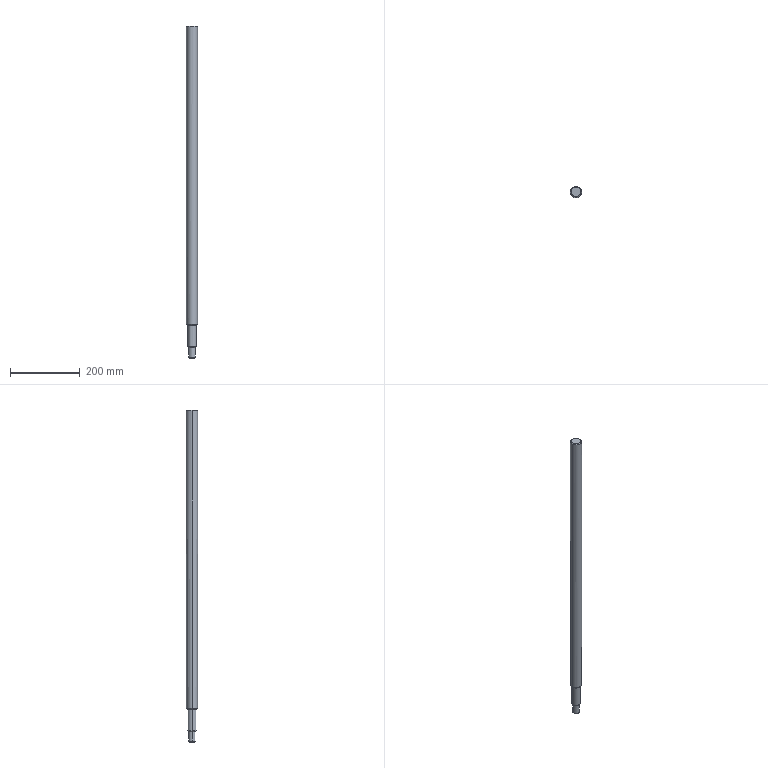Part | SolidWorks | features BaseBody 1, MoveFace 1 | 1 solid | 17 faces | box 32 x 32 x 950.5 mm | volume 728674 mm3 | cone 8 | cylinder 6 | plane 3 | commonest cylinder face diameters 20 x2 25 x2 32 x2
STEP:
#1=CARTESIAN_POINT('',(-16.,0.,948.));
#2=VERTEX_POINT('',#1);
#3=CARTESIAN_POINT('',(16.,0.,948.));
#4=VERTEX_POINT('',#3);
#5=CARTESIAN_POINT('',(0.,0.,948.));
#6=DIRECTION('',(0.,0.,-1.));
#7=DIRECTION('',(-1.,0.,0.));
#8=AXIS2_PLACEMENT_3D('',#5,#6,#7);
#9=CIRCLE('',#8,16.);
#10=EDGE_CURVE('',#2,#4,#9,.T.);
#11=ORIENTED_EDGE('',*,*,#10,.T.);
#12=CARTESIAN_POINT('',(16.,0.,96.5));
#13=VERTEX_POINT('',#12);
#14=CARTESIAN_POINT('',(16.,0.,664.));
#15=DIRECTION('',(0.,0.,-1.));
#16=VECTOR('',#15,1000.);
#17=LINE('',#14,#16);
#18=EDGE_CURVE('',#4,#13,#17,.T.);
#19=ORIENTED_EDGE('',*,*,#18,.T.);
#20=CARTESIAN_POINT('',(0.,16.,96.5));
#21=VERTEX_POINT('',#20);
#22=CARTESIAN_POINT('',(0.,0.,96.5));
#23=DIRECTION('',(0.,0.,1.));
#24=DIRECTION('',(-1.,0.,0.));
#25=AXIS2_PLACEMENT_3D('',#22,#23,#24);
#26=CIRCLE('',#25,16.);
#27=EDGE_CURVE('',#13,#21,#26,.T.);
#28=ORIENTED_EDGE('',*,*,#27,.T.);
#29=CARTESIAN_POINT('',(-16.,0.,96.5));
#30=VERTEX_POINT('',#29);
#31=CARTESIAN_POINT('',(0.,0.,96.5));
#32=DIRECTION('',(0.,0.,1.));
#33=DIRECTION('',(-1.,0.,0.));
#34=AXIS2_PLACEMENT_3D('',#31,#32,#33);
#35=CIRCLE('',#34,16.);
#36=EDGE_CURVE('',#21,#30,#35,.T.);
#37=ORIENTED_EDGE('',*,*,#36,.T.);
#38=CARTESIAN_POINT('',(-16.,0.,664.));
#39=DIRECTION('',(0.,0.,-1.));
#40=VECTOR('',#39,1000.);
#41=LINE('',#38,#40);
#42=EDGE_CURVE('',#2,#30,#41,.T.);
#43=ORIENTED_EDGE('',*,*,#42,.F.);
#44=EDGE_LOOP('',(#11,#19,#28,#37,#43));
#45=FACE_OUTER_BOUND('',#44,.T.);
#46=CARTESIAN_POINT('',(0.,0.,664.));
#47=DIRECTION('',(0.,0.,-1.));
#48=DIRECTION('',(-1.,0.,0.));
#49=AXIS2_PLACEMENT_3D('',#46,#47,#48);
#50=CYLINDRICAL_SURFACE('',#49,16.);
#51=ADVANCED_FACE('',(#45),#50,.T.);
#52=CARTESIAN_POINT('',(0.,-13.5,94.));
#53=VERTEX_POINT('',#52);
#54=CARTESIAN_POINT('',(0.,13.5,94.));
#55=VERTEX_POINT('',#54);
#56=CARTESIAN_POINT('',(0.,0.,94.));
#57=DIRECTION('',(0.,0.,1.));
#58=DIRECTION('',(0.,-1.,0.));
#59=AXIS2_PLACEMENT_3D('',#56,#57,#58);
#60=CIRCLE('',#59,13.5);
#61=EDGE_CURVE('',#53,#55,#60,.T.);
#62=ORIENTED_EDGE('',*,*,#61,.T.);
#63=CARTESIAN_POINT('',(0.,16.,96.5));
#64=DIRECTION('',(0.,0.7071,0.7071));
#65=VECTOR('',#64,1000.);
#66=LINE('',#63,#65);
#67=EDGE_CURVE('',#55,#21,#66,.T.);
#68=ORIENTED_EDGE('',*,*,#67,.T.);
#69=ORIENTED_EDGE('',*,*,#27,.F.);
#70=CARTESIAN_POINT('',(0.,-16.,96.5));
#71=VERTEX_POINT('',#70);
#72=CARTESIAN_POINT('',(0.,0.,96.5));
#73=DIRECTION('',(0.,0.,1.));
#74=DIRECTION('',(-1.,0.,0.));
#75=AXIS2_PLACEMENT_3D('',#72,#73,#74);
#76=CIRCLE('',#75,16.);
#77=EDGE_CURVE('',#71,#13,#76,.T.);
#78=ORIENTED_EDGE('',*,*,#77,.F.);
#79=CARTESIAN_POINT('',(0.,-16.,96.5));
#80=DIRECTION('',(0.,-0.7071,0.7071));
#81=VECTOR('',#80,1000.);
#82=LINE('',#79,#81);
#83=EDGE_CURVE('',#53,#71,#82,.T.);
#84=ORIENTED_EDGE('',*,*,#83,.F.);
#85=EDGE_LOOP('',(#62,#68,#69,#78,#84));
#86=FACE_OUTER_BOUND('',#85,.T.);
#87=CARTESIAN_POINT('',(0.,0.,96.5));
#88=DIRECTION('',(0.,0.,1.));
#89=DIRECTION('',(0.,-1.,0.));
#90=AXIS2_PLACEMENT_3D('',#87,#88,#89);
#91=CONICAL_SURFACE('',#90,16.,0.7854);
#92=ADVANCED_FACE('',(#86),#91,.T.);
#93=CARTESIAN_POINT('',(-13.5,0.,950.5));
#94=VERTEX_POINT('',#93);
#95=CARTESIAN_POINT('',(13.5,0.,950.5));
#96=VERTEX_POINT('',#95);
#97=CARTESIAN_POINT('',(0.,0.,950.5));
#98=DIRECTION('',(0.,0.,-1.));
#99=DIRECTION('',(-1.,0.,0.));
#100=AXIS2_PLACEMENT_3D('',#97,#98,#99);
#101=CIRCLE('',#100,13.5);
#102=EDGE_CURVE('',#94,#96,#101,.T.);
#103=ORIENTED_EDGE('',*,*,#102,.T.);
#104=CARTESIAN_POINT('',(16.,0.,948.));
#105=DIRECTION('',(0.7071,0.,-0.7071));
#106=VECTOR('',#105,1000.);
#107=LINE('',#104,#106);
#108=EDGE_CURVE('',#96,#4,#107,.T.);
#109=ORIENTED_EDGE('',*,*,#108,.T.);
#110=ORIENTED_EDGE('',*,*,#10,.F.);
#111=CARTESIAN_POINT('',(-16.,0.,948.));
#112=DIRECTION('',(-0.7071,0.,-0.7071));
#113=VECTOR('',#112,1000.);
#114=LINE('',#111,#113);
#115=EDGE_CURVE('',#94,#2,#114,.T.);
#116=ORIENTED_EDGE('',*,*,#115,.F.);
#117=EDGE_LOOP('',(#103,#109,#110,#116));
#118=FACE_OUTER_BOUND('',#117,.T.);
#119=CARTESIAN_POINT('',(0.,0.,948.));
#120=DIRECTION('',(0.,0.,-1.));
#121=DIRECTION('',(-1.,0.,0.));
#122=AXIS2_PLACEMENT_3D('',#119,#120,#121);
#123=CONICAL_SURFACE('',#122,16.,0.7854);
#124=ADVANCED_FACE('',(#118),#123,.T.);
#125=CARTESIAN_POINT('',(-12.5,0.,94.));
#126=VERTEX_POINT('',#125);
#127=CARTESIAN_POINT('',(12.5,0.,94.));
#128=VERTEX_POINT('',#127);
#129=CARTESIAN_POINT('',(0.,0.,94.));
#130=DIRECTION('',(0.,0.,-1.));
#131=DIRECTION('',(-1.,0.,0.));
#132=AXIS2_PLACEMENT_3D('',#129,#130,#131);
#133=CIRCLE('',#132,12.5);
#134=EDGE_CURVE('',#126,#128,#133,.T.);
#135=ORIENTED_EDGE('',*,*,#134,.T.);
#136=CARTESIAN_POINT('',(12.5,0.,32.5));
#137=VERTEX_POINT('',#136);
#138=CARTESIAN_POINT('',(12.5,0.,94.));
#139=DIRECTION('',(0.,0.,-1.));
#140=VECTOR('',#139,1000.);
#141=LINE('',#138,#140);
#142=EDGE_CURVE('',#128,#137,#141,.T.);
#143=ORIENTED_EDGE('',*,*,#142,.T.);
#144=CARTESIAN_POINT('',(-12.5,0.,32.5));
#145=VERTEX_POINT('',#144);
#146=CARTESIAN_POINT('',(0.,0.,32.5));
#147=DIRECTION('',(0.,0.,1.));
#148=DIRECTION('',(-1.,0.,0.));
#149=AXIS2_PLACEMENT_3D('',#146,#147,#148);
#150=CIRCLE('',#149,12.5);
#151=EDGE_CURVE('',#137,#145,#150,.T.);
#152=ORIENTED_EDGE('',*,*,#151,.T.);
#153=CARTESIAN_POINT('',(-12.5,0.,94.));
#154=DIRECTION('',(0.,0.,-1.));
#155=VECTOR('',#154,1000.);
#156=LINE('',#153,#155);
#157=EDGE_CURVE('',#126,#145,#156,.T.);
#158=ORIENTED_EDGE('',*,*,#157,.F.);
#159=EDGE_LOOP('',(#135,#143,#152,#158));
#160=FACE_OUTER_BOUND('',#159,.T.);
#161=CARTESIAN_POINT('',(0.,0.,94.));
#162=DIRECTION('',(0.,0.,-1.));
#163=DIRECTION('',(-1.,0.,0.));
#164=AXIS2_PLACEMENT_3D('',#161,#162,#163);
#165=CYLINDRICAL_SURFACE('',#164,12.5);
#166=ADVANCED_FACE('',(#160),#165,.T.);
#167=CARTESIAN_POINT('',(10.,0.,30.));
#168=VERTEX_POINT('',#167);
#169=CARTESIAN_POINT('',(-10.,0.,30.));
#170=VERTEX_POINT('',#169);
#171=CARTESIAN_POINT('',(0.,0.,30.));
#172=DIRECTION('',(0.,0.,1.));
#173=DIRECTION('',(-1.,0.,0.));
#174=AXIS2_PLACEMENT_3D('',#171,#172,#173);
#175=CIRCLE('',#174,10.);
#176=EDGE_CURVE('',#168,#170,#175,.T.);
#177=ORIENTED_EDGE('',*,*,#176,.T.);
#178=CARTESIAN_POINT('',(-12.5,0.,32.5));
#179=DIRECTION('',(-0.7071,0.,0.7071));
#180=VECTOR('',#179,1000.);
#181=LINE('',#178,#180);
#182=EDGE_CURVE('',#170,#145,#181,.T.);
#183=ORIENTED_EDGE('',*,*,#182,.T.);
#184=ORIENTED_EDGE('',*,*,#151,.F.);
#185=CARTESIAN_POINT('',(12.5,0.,32.5));
#186=DIRECTION('',(0.7071,0.,0.7071));
#187=VECTOR('',#186,1000.);
#188=LINE('',#185,#187);
#189=EDGE_CURVE('',#168,#137,#188,.T.);
#190=ORIENTED_EDGE('',*,*,#189,.F.);
#191=EDGE_LOOP('',(#177,#183,#184,#190));
#192=FACE_OUTER_BOUND('',#191,.T.);
#193=CARTESIAN_POINT('',(0.,0.,32.5));
#194=DIRECTION('',(0.,0.,1.));
#195=DIRECTION('',(1.,0.,0.));
#196=AXIS2_PLACEMENT_3D('',#193,#194,#195);
#197=CONICAL_SURFACE('',#196,12.5,0.7854);
#198=ADVANCED_FACE('',(#192),#197,.T.);
#199=ORIENTED_EDGE('',*,*,#176,.F.);
#200=CARTESIAN_POINT('',(10.,0.,2.5));
#201=VERTEX_POINT('',#200);
#202=CARTESIAN_POINT('',(10.,0.,30.));
#203=DIRECTION('',(0.,0.,-1.));
#204=VECTOR('',#203,1000.);
#205=LINE('',#202,#204);
#206=EDGE_CURVE('',#168,#201,#205,.T.);
#207=ORIENTED_EDGE('',*,*,#206,.T.);
#208=CARTESIAN_POINT('',(-10.,0.,2.5));
#209=VERTEX_POINT('',#208);
#210=CARTESIAN_POINT('',(0.,0.,2.5));
#211=DIRECTION('',(0.,0.,1.));
#212=DIRECTION('',(-1.,0.,0.));
#213=AXIS2_PLACEMENT_3D('',#210,#211,#212);
#214=CIRCLE('',#213,10.);
#215=EDGE_CURVE('',#201,#209,#214,.T.);
#216=ORIENTED_EDGE('',*,*,#215,.T.);
#217=CARTESIAN_POINT('',(-10.,0.,30.));
#218=DIRECTION('',(0.,0.,-1.));
#219=VECTOR('',#218,1000.);
#220=LINE('',#217,#219);
#221=EDGE_CURVE('',#170,#209,#220,.T.);
#222=ORIENTED_EDGE('',*,*,#221,.F.);
#223=EDGE_LOOP('',(#199,#207,#216,#222));
#224=FACE_OUTER_BOUND('',#223,.T.);
#225=CARTESIAN_POINT('',(0.,0.,30.));
#226=DIRECTION('',(0.,0.,-1.));
#227=DIRECTION('',(-1.,0.,0.));
#228=AXIS2_PLACEMENT_3D('',#225,#226,#227);
#229=CYLINDRICAL_SURFACE('',#228,10.);
#230=ADVANCED_FACE('',(#224),#229,.T.);
#231=CARTESIAN_POINT('',(7.5,0.,0.));
#232=VERTEX_POINT('',#231);
#233=CARTESIAN_POINT('',(-7.5,0.,0.));
#234=VERTEX_POINT('',#233);
#235=CARTESIAN_POINT('',(0.,0.,0.));
#236=DIRECTION('',(0.,0.,1.));
#237=DIRECTION('',(1.,0.,0.));
#238=AXIS2_PLACEMENT_3D('',#235,#236,#237);
#239=CIRCLE('',#238,7.5);
#240=EDGE_CURVE('',#232,#234,#239,.T.);
#241=ORIENTED_EDGE('',*,*,#240,.T.);
#242=CARTESIAN_POINT('',(-10.,0.,2.5));
#243=DIRECTION('',(-0.7071,0.,0.7071));
#244=VECTOR('',#243,1000.);
#245=LINE('',#242,#244);
#246=EDGE_CURVE('',#234,#209,#245,.T.);
#247=ORIENTED_EDGE('',*,*,#246,.T.);
#248=ORIENTED_EDGE('',*,*,#215,.F.);
#249=CARTESIAN_POINT('',(10.,0.,2.5));
#250=DIRECTION('',(0.7071,0.,0.7071));
#251=VECTOR('',#250,1000.);
#252=LINE('',#249,#251);
#253=EDGE_CURVE('',#232,#201,#252,.T.);
#254=ORIENTED_EDGE('',*,*,#253,.F.);
#255=EDGE_LOOP('',(#241,#247,#248,#254));
#256=FACE_OUTER_BOUND('',#255,.T.);
#257=CARTESIAN_POINT('',(0.,0.,2.5));
#258=DIRECTION('',(0.,0.,1.));
#259=DIRECTION('',(1.,0.,0.));
#260=AXIS2_PLACEMENT_3D('',#257,#258,#259);
#261=CONICAL_SURFACE('',#260,10.,0.7854);
#262=ADVANCED_FACE('',(#256),#261,.T.);
#263=ORIENTED_EDGE('',*,*,#18,.F.);
#264=CARTESIAN_POINT('',(0.,0.,948.));
#265=DIRECTION('',(0.,0.,-1.));
#266=DIRECTION('',(-1.,0.,0.));
#267=AXIS2_PLACEMENT_3D('',#264,#265,#266);
#268=CIRCLE('',#267,16.);
#269=EDGE_CURVE('',#4,#2,#268,.T.);
#270=ORIENTED_EDGE('',*,*,#269,.T.);
#271=ORIENTED_EDGE('',*,*,#42,.T.);
#272=CARTESIAN_POINT('',(0.,0.,96.5));
#273=DIRECTION('',(0.,0.,1.));
#274=DIRECTION('',(-1.,0.,0.));
#275=AXIS2_PLACEMENT_3D('',#272,#273,#274);
#276=CIRCLE('',#275,16.);
#277=EDGE_CURVE('',#30,#71,#276,.T.);
#278=ORIENTED_EDGE('',*,*,#277,.T.);
#279=ORIENTED_EDGE('',*,*,#77,.T.);
#280=EDGE_LOOP('',(#263,#270,#271,#278,#279));
#281=FACE_OUTER_BOUND('',#280,.T.);
#282=CARTESIAN_POINT('',(0.,0.,664.));
#283=DIRECTION('',(0.,0.,-1.));
#284=DIRECTION('',(-1.,0.,0.));
#285=AXIS2_PLACEMENT_3D('',#282,#283,#284);
#286=CYLINDRICAL_SURFACE('',#285,16.);
#287=ADVANCED_FACE('',(#281),#286,.T.);
#288=ORIENTED_EDGE('',*,*,#67,.F.);
#289=CARTESIAN_POINT('',(0.,0.,94.));
#290=DIRECTION('',(0.,0.,1.));
#291=DIRECTION('',(0.,-1.,0.));
#292=AXIS2_PLACEMENT_3D('',#289,#290,#291);
#293=CIRCLE('',#292,13.5);
#294=EDGE_CURVE('',#55,#53,#293,.T.);
#295=ORIENTED_EDGE('',*,*,#294,.T.);
#296=ORIENTED_EDGE('',*,*,#83,.T.);
#297=ORIENTED_EDGE('',*,*,#277,.F.);
#298=ORIENTED_EDGE('',*,*,#36,.F.);
#299=EDGE_LOOP('',(#288,#295,#296,#297,#298));
#300=FACE_OUTER_BOUND('',#299,.T.);
#301=CARTESIAN_POINT('',(0.,0.,96.5));
#302=DIRECTION('',(0.,0.,1.));
#303=DIRECTION('',(0.,-1.,0.));
#304=AXIS2_PLACEMENT_3D('',#301,#302,#303);
#305=CONICAL_SURFACE('',#304,16.,0.7854);
#306=ADVANCED_FACE('',(#300),#305,.T.);
#307=ORIENTED_EDGE('',*,*,#108,.F.);
#308=CARTESIAN_POINT('',(0.,0.,950.5));
#309=DIRECTION('',(0.,0.,-1.));
#310=DIRECTION('',(-1.,0.,0.));
#311=AXIS2_PLACEMENT_3D('',#308,#309,#310);
#312=CIRCLE('',#311,13.5);
#313=EDGE_CURVE('',#96,#94,#312,.T.);
#314=ORIENTED_EDGE('',*,*,#313,.T.);
#315=ORIENTED_EDGE('',*,*,#115,.T.);
#316=ORIENTED_EDGE('',*,*,#269,.F.);
#317=EDGE_LOOP('',(#307,#314,#315,#316));
#318=FACE_OUTER_BOUND('',#317,.T.);
#319=CARTESIAN_POINT('',(0.,0.,948.));
#320=DIRECTION('',(0.,0.,-1.));
#321=DIRECTION('',(-1.,0.,0.));
#322=AXIS2_PLACEMENT_3D('',#319,#320,#321);
#323=CONICAL_SURFACE('',#322,16.,0.7854);
#324=ADVANCED_FACE('',(#318),#323,.T.);
#325=ORIENTED_EDGE('',*,*,#134,.F.);
#326=CARTESIAN_POINT('',(0.,0.,94.));
#327=DIRECTION('',(0.,0.,-1.));
#328=DIRECTION('',(-1.,0.,0.));
#329=AXIS2_PLACEMENT_3D('',#326,#327,#328);
#330=CIRCLE('',#329,12.5);
#331=EDGE_CURVE('',#128,#126,#330,.T.);
#332=ORIENTED_EDGE('',*,*,#331,.F.);
#333=EDGE_LOOP('',(#325,#332));
#334=FACE_BOUND('',#333,.T.);
#335=ORIENTED_EDGE('',*,*,#61,.F.);
#336=ORIENTED_EDGE('',*,*,#294,.F.);
#337=EDGE_LOOP('',(#335,#336));
#338=FACE_OUTER_BOUND('',#337,.T.);
#339=CARTESIAN_POINT('',(0.,0.,94.));
#340=DIRECTION('',(0.,0.,1.));
#341=DIRECTION('',(1.,0.,0.));
#342=AXIS2_PLACEMENT_3D('',#339,#340,#341);
#343=PLANE('',#342);
#344=ADVANCED_FACE('',(#334,#338),#343,.F.);
#345=ORIENTED_EDGE('',*,*,#102,.F.);
#346=ORIENTED_EDGE('',*,*,#313,.F.);
#347=EDGE_LOOP('',(#345,#346));
#348=FACE_OUTER_BOUND('',#347,.T.);
#349=CARTESIAN_POINT('',(0.,0.,950.5));
#350=DIRECTION('',(0.,0.,1.));
#351=DIRECTION('',(1.,0.,0.));
#352=AXIS2_PLACEMENT_3D('',#349,#350,#351);
#353=PLANE('',#352);
#354=ADVANCED_FACE('',(#348),#353,.T.);
#355=ORIENTED_EDGE('',*,*,#142,.F.);
#356=ORIENTED_EDGE('',*,*,#331,.T.);
#357=ORIENTED_EDGE('',*,*,#157,.T.);
#358=CARTESIAN_POINT('',(0.,0.,32.5));
#359=DIRECTION('',(0.,0.,1.));
#360=DIRECTION('',(-1.,0.,0.));
#361=AXIS2_PLACEMENT_3D('',#358,#359,#360);
#362=CIRCLE('',#361,12.5);
#363=EDGE_CURVE('',#145,#137,#362,.T.);
#364=ORIENTED_EDGE('',*,*,#363,.T.);
#365=EDGE_LOOP('',(#355,#356,#357,#364));
#366=FACE_OUTER_BOUND('',#365,.T.);
#367=CARTESIAN_POINT('',(0.,0.,94.));
#368=DIRECTION('',(0.,0.,-1.));
#369=DIRECTION('',(-1.,0.,0.));
#370=AXIS2_PLACEMENT_3D('',#367,#368,#369);
#371=CYLINDRICAL_SURFACE('',#370,12.5);
#372=ADVANCED_FACE('',(#366),#371,.T.);
#373=ORIENTED_EDGE('',*,*,#182,.F.);
#374=CARTESIAN_POINT('',(0.,0.,30.));
#375=DIRECTION('',(0.,0.,1.));
#376=DIRECTION('',(-1.,0.,0.));
#377=AXIS2_PLACEMENT_3D('',#374,#375,#376);
#378=CIRCLE('',#377,10.);
#379=EDGE_CURVE('',#170,#168,#378,.T.);
#380=ORIENTED_EDGE('',*,*,#379,.T.);
#381=ORIENTED_EDGE('',*,*,#189,.T.);
#382=ORIENTED_EDGE('',*,*,#363,.F.);
#383=EDGE_LOOP('',(#373,#380,#381,#382));
#384=FACE_OUTER_BOUND('',#383,.T.);
#385=CARTESIAN_POINT('',(0.,0.,32.5));
#386=DIRECTION('',(0.,0.,1.));
#387=DIRECTION('',(1.,0.,0.));
#388=AXIS2_PLACEMENT_3D('',#385,#386,#387);
#389=CONICAL_SURFACE('',#388,12.5,0.7854);
#390=ADVANCED_FACE('',(#384),#389,.T.);
#391=ORIENTED_EDGE('',*,*,#206,.F.);
#392=ORIENTED_EDGE('',*,*,#379,.F.);
#393=ORIENTED_EDGE('',*,*,#221,.T.);
#394=CARTESIAN_POINT('',(0.,0.,2.5));
#395=DIRECTION('',(0.,0.,1.));
#396=DIRECTION('',(-1.,0.,0.));
#397=AXIS2_PLACEMENT_3D('',#394,#395,#396);
#398=CIRCLE('',#397,10.);
#399=EDGE_CURVE('',#209,#201,#398,.T.);
#400=ORIENTED_EDGE('',*,*,#399,.T.);
#401=EDGE_LOOP('',(#391,#392,#393,#400));
#402=FACE_OUTER_BOUND('',#401,.T.);
#403=CARTESIAN_POINT('',(0.,0.,30.));
#404=DIRECTION('',(0.,0.,-1.));
#405=DIRECTION('',(-1.,0.,0.));
#406=AXIS2_PLACEMENT_3D('',#403,#404,#405);
#407=CYLINDRICAL_SURFACE('',#406,10.);
#408=ADVANCED_FACE('',(#402),#407,.T.);
#409=ORIENTED_EDGE('',*,*,#246,.F.);
#410=CARTESIAN_POINT('',(0.,0.,0.));
#411=DIRECTION('',(0.,0.,1.));
#412=DIRECTION('',(1.,0.,0.));
#413=AXIS2_PLACEMENT_3D('',#410,#411,#412);
#414=CIRCLE('',#413,7.5);
#415=EDGE_CURVE('',#234,#232,#414,.T.);
#416=ORIENTED_EDGE('',*,*,#415,.T.);
#417=ORIENTED_EDGE('',*,*,#253,.T.);
#418=ORIENTED_EDGE('',*,*,#399,.F.);
#419=EDGE_LOOP('',(#409,#416,#417,#418));
#420=FACE_OUTER_BOUND('',#419,.T.);
#421=CARTESIAN_POINT('',(0.,0.,2.5));
#422=DIRECTION('',(0.,0.,1.));
#423=DIRECTION('',(1.,0.,0.));
#424=AXIS2_PLACEMENT_3D('',#421,#422,#423);
#425=CONICAL_SURFACE('',#424,10.,0.7854);
#426=ADVANCED_FACE('',(#420),#425,.T.);
#427=ORIENTED_EDGE('',*,*,#240,.F.);
#428=ORIENTED_EDGE('',*,*,#415,.F.);
#429=EDGE_LOOP('',(#427,#428));
#430=FACE_OUTER_BOUND('',#429,.T.);
#431=CARTESIAN_POINT('',(0.,0.,0.));
#432=DIRECTION('',(0.,0.,1.));
#433=DIRECTION('',(1.,0.,0.));
#434=AXIS2_PLACEMENT_3D('',#431,#432,#433);
#435=PLANE('',#434);
#436=ADVANCED_FACE('',(#430),#435,.F.);
#437=CLOSED_SHELL('',(#51,#92,#124,#166,#198,#230,#262,#287,#306,#324,#344,#354,#372,#390,#408,#426,#436));
#438=MANIFOLD_SOLID_BREP('',#437);
#439=CARTESIAN_POINT('',(0.,0.,0.));
#440=DIRECTION('',(0.,0.,1.));
#441=DIRECTION('',(1.,0.,0.));
#442=AXIS2_PLACEMENT_3D('',#439,#440,#441);
#443=(LENGTH_UNIT()NAMED_UNIT(*)SI_UNIT(.MILLI.,.METRE.));
#444=UNCERTAINTY_MEASURE_WITH_UNIT(LENGTH_MEASURE(0.00001),#443,'','');
#445=(NAMED_UNIT(*)PLANE_ANGLE_UNIT()SI_UNIT($,.RADIAN.));
#446=(NAMED_UNIT(*)SI_UNIT($,.STERADIAN.)SOLID_ANGLE_UNIT());
#447=(GEOMETRIC_REPRESENTATION_CONTEXT(3)GLOBAL_UNCERTAINTY_ASSIGNED_CONTEXT((#444))GLOBAL_UNIT_ASSIGNED_CONTEXT((#443,#445,#446))REPRESENTATION_CONTEXT('',''));
#448=ADVANCED_BREP_SHAPE_REPRESENTATION('',(#438,#442),#447);